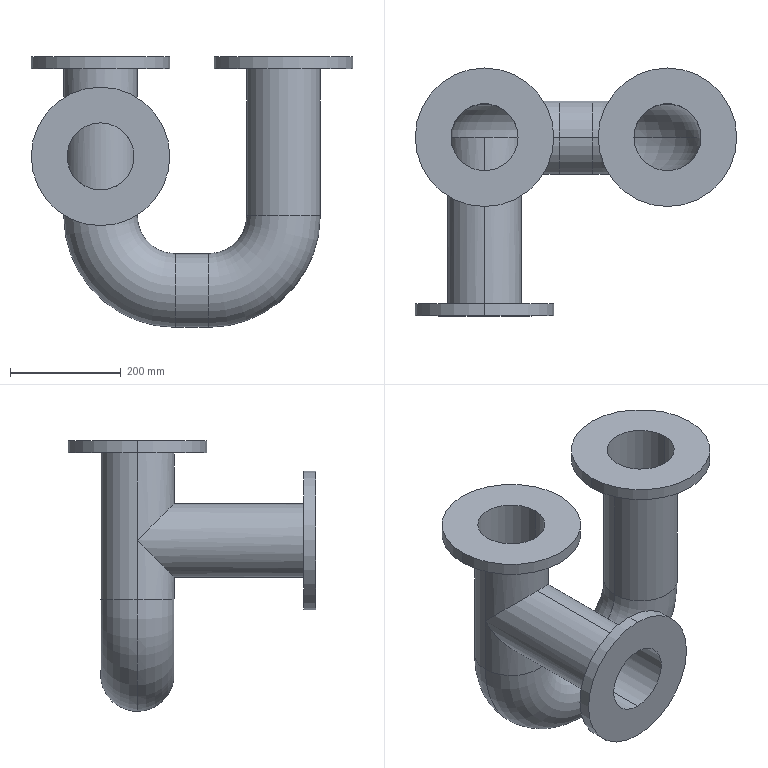Part | SolidWorks | features ICE 3, 3DProfileFeature 1, HoleWzd 1, Sweep 1 | 1 solid | 50 faces | box 580 x 447 x 488.5 mm | volume 5598640 mm3 | cylinder 34 | torus 8 | plane 8 | commonest cylinder face diameters 121 x13 133 x13 250 x6 14 x2